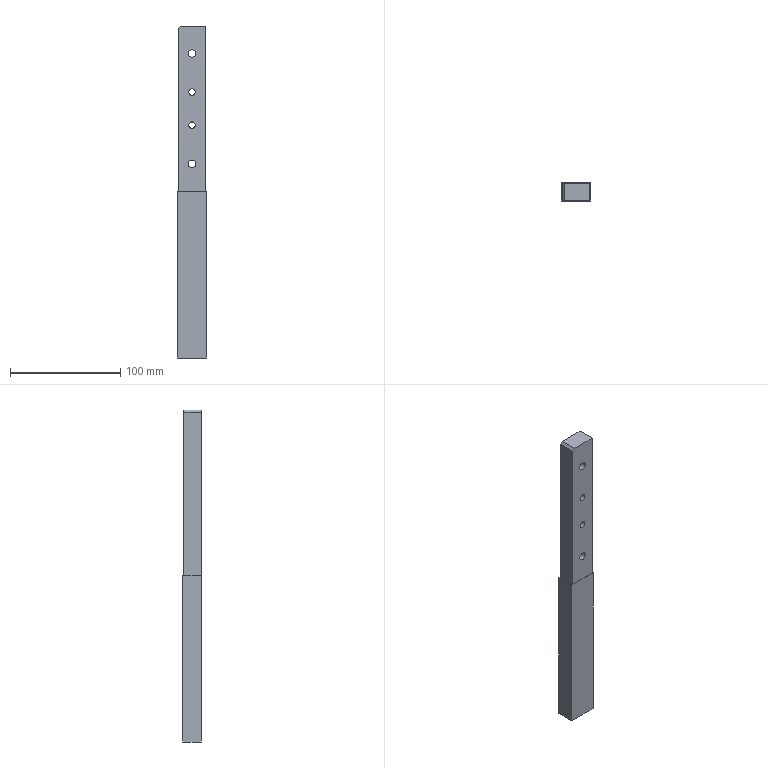Part | NX | features BREP 2 | 2 solids | 25 faces | box 27 x 16.6 x 301 mm | volume 123108 mm3 | plane 17 | cylinder 8 | commonest cylinder face diameters 7 x4 6 x2 11 x2
STEP:
#1=CARTESIAN_POINT('',(26.,16.6,0.));
#2=VERTEX_POINT('',#1);
#3=CARTESIAN_POINT('',(26.,0.,0.));
#4=VERTEX_POINT('',#3);
#5=CARTESIAN_POINT('',(26.,15.6,0.));
#6=DIRECTION('',(0.,-1.,0.));
#7=VECTOR('',#6,1000.);
#8=LINE('',#5,#7);
#9=EDGE_CURVE('',#2,#4,#8,.T.);
#10=ORIENTED_EDGE('',*,*,#9,.T.);
#11=CARTESIAN_POINT('',(26.,0.,-151.));
#12=VERTEX_POINT('',#11);
#13=CARTESIAN_POINT('',(26.,0.,-151.));
#14=DIRECTION('',(0.,0.,1.));
#15=VECTOR('',#14,1000.);
#16=LINE('',#13,#15);
#17=EDGE_CURVE('',#12,#4,#16,.T.);
#18=ORIENTED_EDGE('',*,*,#17,.F.);
#19=CARTESIAN_POINT('',(26.,16.6,-151.));
#20=VERTEX_POINT('',#19);
#21=CARTESIAN_POINT('',(26.,15.6,-151.));
#22=DIRECTION('',(0.,-1.,0.));
#23=VECTOR('',#22,1000.);
#24=LINE('',#21,#23);
#25=EDGE_CURVE('',#20,#12,#24,.T.);
#26=ORIENTED_EDGE('',*,*,#25,.F.);
#27=CARTESIAN_POINT('',(26.,16.6,-151.));
#28=DIRECTION('',(0.,0.,1.));
#29=VECTOR('',#28,1000.);
#30=LINE('',#27,#29);
#31=EDGE_CURVE('',#20,#2,#30,.T.);
#32=ORIENTED_EDGE('',*,*,#31,.T.);
#33=EDGE_LOOP('',(#10,#18,#26,#32));
#34=FACE_BOUND('',#33,.T.);
#35=CARTESIAN_POINT('',(26.,15.6,-151.));
#36=DIRECTION('',(-1.,0.,0.));
#37=DIRECTION('',(0.,1.,0.));
#38=AXIS2_PLACEMENT_3D('',#35,#36,#37);
#39=PLANE('',#38);
#40=ADVANCED_FACE('',(#34),#39,.F.);
#41=CARTESIAN_POINT('',(-1.,0.,0.));
#42=VERTEX_POINT('',#41);
#43=CARTESIAN_POINT('',(25.,0.,0.));
#44=DIRECTION('',(-1.,0.,0.));
#45=VECTOR('',#44,1000.);
#46=LINE('',#43,#45);
#47=EDGE_CURVE('',#4,#42,#46,.T.);
#48=ORIENTED_EDGE('',*,*,#47,.T.);
#49=CARTESIAN_POINT('',(-1.,0.,-151.));
#50=VERTEX_POINT('',#49);
#51=CARTESIAN_POINT('',(-1.,0.,-151.));
#52=DIRECTION('',(0.,0.,1.));
#53=VECTOR('',#52,1000.);
#54=LINE('',#51,#53);
#55=EDGE_CURVE('',#50,#42,#54,.T.);
#56=ORIENTED_EDGE('',*,*,#55,.F.);
#57=CARTESIAN_POINT('',(25.,0.,-151.));
#58=DIRECTION('',(-1.,0.,0.));
#59=VECTOR('',#58,1000.);
#60=LINE('',#57,#59);
#61=EDGE_CURVE('',#12,#50,#60,.T.);
#62=ORIENTED_EDGE('',*,*,#61,.F.);
#63=ORIENTED_EDGE('',*,*,#17,.T.);
#64=EDGE_LOOP('',(#48,#56,#62,#63));
#65=FACE_BOUND('',#64,.T.);
#66=CARTESIAN_POINT('',(25.,0.,-151.));
#67=DIRECTION('',(0.,1.,0.));
#68=DIRECTION('',(1.,0.,0.));
#69=AXIS2_PLACEMENT_3D('',#66,#67,#68);
#70=PLANE('',#69);
#71=ADVANCED_FACE('',(#65),#70,.F.);
#72=CARTESIAN_POINT('',(-1.,16.6,0.));
#73=VERTEX_POINT('',#72);
#74=CARTESIAN_POINT('',(-1.,10.6,0.));
#75=DIRECTION('',(0.,1.,0.));
#76=VECTOR('',#75,1000.);
#77=LINE('',#74,#76);
#78=EDGE_CURVE('',#42,#73,#77,.T.);
#79=ORIENTED_EDGE('',*,*,#78,.T.);
#80=CARTESIAN_POINT('',(-1.,16.6,-151.));
#81=VERTEX_POINT('',#80);
#82=CARTESIAN_POINT('',(-1.,16.6,-151.));
#83=DIRECTION('',(0.,0.,1.));
#84=VECTOR('',#83,1000.);
#85=LINE('',#82,#84);
#86=EDGE_CURVE('',#81,#73,#85,.T.);
#87=ORIENTED_EDGE('',*,*,#86,.F.);
#88=CARTESIAN_POINT('',(-1.,10.6,-151.));
#89=DIRECTION('',(0.,1.,0.));
#90=VECTOR('',#89,1000.);
#91=LINE('',#88,#90);
#92=EDGE_CURVE('',#50,#81,#91,.T.);
#93=ORIENTED_EDGE('',*,*,#92,.F.);
#94=ORIENTED_EDGE('',*,*,#55,.T.);
#95=EDGE_LOOP('',(#79,#87,#93,#94));
#96=FACE_BOUND('',#95,.T.);
#97=CARTESIAN_POINT('',(-1.,10.6,-151.));
#98=DIRECTION('',(1.,0.,0.));
#99=DIRECTION('',(0.,0.,1.));
#100=AXIS2_PLACEMENT_3D('',#97,#98,#99);
#101=PLANE('',#100);
#102=ADVANCED_FACE('',(#96),#101,.F.);
#103=CARTESIAN_POINT('',(0.,16.6,0.));
#104=DIRECTION('',(1.,0.,0.));
#105=VECTOR('',#104,1000.);
#106=LINE('',#103,#105);
#107=EDGE_CURVE('',#73,#2,#106,.T.);
#108=ORIENTED_EDGE('',*,*,#107,.T.);
#109=ORIENTED_EDGE('',*,*,#31,.F.);
#110=CARTESIAN_POINT('',(0.,16.6,-151.));
#111=DIRECTION('',(1.,0.,0.));
#112=VECTOR('',#111,1000.);
#113=LINE('',#110,#112);
#114=EDGE_CURVE('',#81,#20,#113,.T.);
#115=ORIENTED_EDGE('',*,*,#114,.F.);
#116=ORIENTED_EDGE('',*,*,#86,.T.);
#117=EDGE_LOOP('',(#108,#109,#115,#116));
#118=FACE_BOUND('',#117,.T.);
#119=CARTESIAN_POINT('',(0.,16.6,-151.));
#120=DIRECTION('',(0.,-1.,0.));
#121=DIRECTION('',(0.,0.,1.));
#122=AXIS2_PLACEMENT_3D('',#119,#120,#121);
#123=PLANE('',#122);
#124=ADVANCED_FACE('',(#118),#123,.F.);
#125=ORIENTED_EDGE('',*,*,#25,.T.);
#126=ORIENTED_EDGE('',*,*,#61,.T.);
#127=ORIENTED_EDGE('',*,*,#92,.T.);
#128=ORIENTED_EDGE('',*,*,#114,.T.);
#129=EDGE_LOOP('',(#125,#126,#127,#128));
#130=FACE_BOUND('',#129,.T.);
#131=CARTESIAN_POINT('',(25.,0.,-151.));
#132=DIRECTION('',(0.,0.,-1.));
#133=DIRECTION('',(1.,0.,0.));
#134=AXIS2_PLACEMENT_3D('',#131,#132,#133);
#135=PLANE('',#134);
#136=ADVANCED_FACE('',(#130),#135,.T.);
#137=ORIENTED_EDGE('',*,*,#9,.F.);
#138=ORIENTED_EDGE('',*,*,#107,.F.);
#139=ORIENTED_EDGE('',*,*,#78,.F.);
#140=ORIENTED_EDGE('',*,*,#47,.F.);
#141=EDGE_LOOP('',(#137,#138,#139,#140));
#142=FACE_BOUND('',#141,.T.);
#143=CARTESIAN_POINT('',(25.,0.,0.));
#144=DIRECTION('',(0.,0.,-1.));
#145=DIRECTION('',(1.,0.,0.));
#146=AXIS2_PLACEMENT_3D('',#143,#144,#145);
#147=PLANE('',#146);
#148=ADVANCED_FACE('',(#142),#147,.F.);
#149=CLOSED_SHELL('',(#40,#71,#102,#124,#136,#148));
#150=MANIFOLD_SOLID_BREP('',#149);
#151=CARTESIAN_POINT('',(25.,0.,150.));
#152=VERTEX_POINT('',#151);
#153=CARTESIAN_POINT('',(25.,0.,0.));
#154=VERTEX_POINT('',#153);
#155=CARTESIAN_POINT('',(25.,0.,150.));
#156=DIRECTION('',(0.,0.,-1.));
#157=VECTOR('',#156,1000.);
#158=LINE('',#155,#157);
#159=EDGE_CURVE('',#152,#154,#158,.T.);
#160=ORIENTED_EDGE('',*,*,#159,.T.);
#161=CARTESIAN_POINT('',(25.,15.6,0.));
#162=VERTEX_POINT('',#161);
#163=CARTESIAN_POINT('',(25.,15.6,0.));
#164=DIRECTION('',(0.,1.,0.));
#165=VECTOR('',#164,1000.);
#166=LINE('',#163,#165);
#167=EDGE_CURVE('',#154,#162,#166,.T.);
#168=ORIENTED_EDGE('',*,*,#167,.T.);
#169=CARTESIAN_POINT('',(25.,15.6,150.));
#170=VERTEX_POINT('',#169);
#171=CARTESIAN_POINT('',(25.,15.6,150.));
#172=DIRECTION('',(0.,0.,-1.));
#173=VECTOR('',#172,1000.);
#174=LINE('',#171,#173);
#175=EDGE_CURVE('',#170,#162,#174,.T.);
#176=ORIENTED_EDGE('',*,*,#175,.F.);
#177=CARTESIAN_POINT('',(25.,15.6,150.));
#178=DIRECTION('',(0.,-1.,0.));
#179=VECTOR('',#178,1000.);
#180=LINE('',#177,#179);
#181=EDGE_CURVE('',#170,#152,#180,.T.);
#182=ORIENTED_EDGE('',*,*,#181,.T.);
#183=EDGE_LOOP('',(#160,#168,#176,#182));
#184=FACE_BOUND('',#183,.T.);
#185=CARTESIAN_POINT('',(25.,15.6,150.));
#186=DIRECTION('',(1.,0.,0.));
#187=DIRECTION('',(0.,-1.,0.));
#188=AXIS2_PLACEMENT_3D('',#185,#186,#187);
#189=PLANE('',#188);
#190=ADVANCED_FACE('',(#184),#189,.T.);
#191=CARTESIAN_POINT('',(0.,15.6,148.));
#192=VERTEX_POINT('',#191);
#193=CARTESIAN_POINT('',(0.,15.6,0.));
#194=VERTEX_POINT('',#193);
#195=CARTESIAN_POINT('',(0.,15.6,150.));
#196=DIRECTION('',(0.,0.,-1.));
#197=VECTOR('',#196,1000.);
#198=LINE('',#195,#197);
#199=EDGE_CURVE('',#192,#194,#198,.T.);
#200=ORIENTED_EDGE('',*,*,#199,.T.);
#201=CARTESIAN_POINT('',(0.,0.,0.));
#202=VERTEX_POINT('',#201);
#203=CARTESIAN_POINT('',(0.,10.6,0.));
#204=DIRECTION('',(0.,-1.,0.));
#205=VECTOR('',#204,1000.);
#206=LINE('',#203,#205);
#207=EDGE_CURVE('',#194,#202,#206,.T.);
#208=ORIENTED_EDGE('',*,*,#207,.T.);
#209=CARTESIAN_POINT('',(0.,0.,148.));
#210=VERTEX_POINT('',#209);
#211=CARTESIAN_POINT('',(0.,0.,150.));
#212=DIRECTION('',(0.,0.,-1.));
#213=VECTOR('',#212,1000.);
#214=LINE('',#211,#213);
#215=EDGE_CURVE('',#210,#202,#214,.T.);
#216=ORIENTED_EDGE('',*,*,#215,.F.);
#217=CARTESIAN_POINT('',(0.,15.6,148.));
#218=DIRECTION('',(0.,1.,0.));
#219=VECTOR('',#218,1000.);
#220=LINE('',#217,#219);
#221=EDGE_CURVE('',#210,#192,#220,.T.);
#222=ORIENTED_EDGE('',*,*,#221,.T.);
#223=EDGE_LOOP('',(#200,#208,#216,#222));
#224=FACE_BOUND('',#223,.T.);
#225=CARTESIAN_POINT('',(0.,10.6,150.));
#226=DIRECTION('',(-1.,0.,0.));
#227=DIRECTION('',(0.,0.,-1.));
#228=AXIS2_PLACEMENT_3D('',#225,#226,#227);
#229=PLANE('',#228);
#230=ADVANCED_FACE('',(#224),#229,.T.);
#231=CARTESIAN_POINT('',(12.5,15.6,86.5));
#232=VERTEX_POINT('',#231);
#233=CARTESIAN_POINT('',(12.5,15.6,90.));
#234=DIRECTION('',(0.,1.,0.));
#235=DIRECTION('',(0.,0.,-1.));
#236=AXIS2_PLACEMENT_3D('',#233,#234,#235);
#237=CIRCLE('',#236,3.5);
#238=EDGE_CURVE('',#232,#232,#237,.T.);
#239=ORIENTED_EDGE('',*,*,#238,.F.);
#240=EDGE_LOOP('',(#239));
#241=FACE_BOUND('',#240,.T.);
#242=CARTESIAN_POINT('',(12.5,15.6,56.5));
#243=VERTEX_POINT('',#242);
#244=CARTESIAN_POINT('',(12.5,15.6,60.));
#245=DIRECTION('',(0.,1.,0.));
#246=DIRECTION('',(0.,0.,-1.));
#247=AXIS2_PLACEMENT_3D('',#244,#245,#246);
#248=CIRCLE('',#247,3.5);
#249=EDGE_CURVE('',#243,#243,#248,.T.);
#250=ORIENTED_EDGE('',*,*,#249,.F.);
#251=EDGE_LOOP('',(#250));
#252=FACE_BOUND('',#251,.T.);
#253=CARTESIAN_POINT('',(12.5,15.6,119.5));
#254=VERTEX_POINT('',#253);
#255=CARTESIAN_POINT('',(12.5,15.6,125.));
#256=DIRECTION('',(0.,1.,0.));
#257=DIRECTION('',(0.,0.,-1.));
#258=AXIS2_PLACEMENT_3D('',#255,#256,#257);
#259=CIRCLE('',#258,5.5);
#260=EDGE_CURVE('',#254,#254,#259,.T.);
#261=ORIENTED_EDGE('',*,*,#260,.F.);
#262=EDGE_LOOP('',(#261));
#263=FACE_BOUND('',#262,.T.);
#264=CARTESIAN_POINT('',(12.5,15.6,19.5));
#265=VERTEX_POINT('',#264);
#266=CARTESIAN_POINT('',(12.5,15.6,25.));
#267=DIRECTION('',(0.,1.,0.));
#268=DIRECTION('',(0.,0.,-1.));
#269=AXIS2_PLACEMENT_3D('',#266,#267,#268);
#270=CIRCLE('',#269,5.5);
#271=EDGE_CURVE('',#265,#265,#270,.T.);
#272=ORIENTED_EDGE('',*,*,#271,.F.);
#273=EDGE_LOOP('',(#272));
#274=FACE_BOUND('',#273,.T.);
#275=ORIENTED_EDGE('',*,*,#175,.T.);
#276=CARTESIAN_POINT('',(0.,15.6,0.));
#277=DIRECTION('',(-1.,0.,0.));
#278=VECTOR('',#277,1000.);
#279=LINE('',#276,#278);
#280=EDGE_CURVE('',#162,#194,#279,.T.);
#281=ORIENTED_EDGE('',*,*,#280,.T.);
#282=ORIENTED_EDGE('',*,*,#199,.F.);
#283=CARTESIAN_POINT('',(2.,15.6,150.));
#284=VERTEX_POINT('',#283);
#285=CARTESIAN_POINT('',(1.,15.6,149.));
#286=DIRECTION('',(0.7071,0.,0.7071));
#287=VECTOR('',#286,1000.);
#288=LINE('',#285,#287);
#289=EDGE_CURVE('',#192,#284,#288,.T.);
#290=ORIENTED_EDGE('',*,*,#289,.T.);
#291=CARTESIAN_POINT('',(0.,15.6,150.));
#292=DIRECTION('',(1.,0.,0.));
#293=VECTOR('',#292,1000.);
#294=LINE('',#291,#293);
#295=EDGE_CURVE('',#284,#170,#294,.T.);
#296=ORIENTED_EDGE('',*,*,#295,.T.);
#297=EDGE_LOOP('',(#275,#281,#282,#290,#296));
#298=FACE_BOUND('',#297,.T.);
#299=CARTESIAN_POINT('',(0.,15.6,150.));
#300=DIRECTION('',(0.,1.,0.));
#301=DIRECTION('',(0.,0.,-1.));
#302=AXIS2_PLACEMENT_3D('',#299,#300,#301);
#303=PLANE('',#302);
#304=ADVANCED_FACE('',(#241,#252,#263,#274,#298),#303,.T.);
#305=CARTESIAN_POINT('',(15.5,0.,90.));
#306=VERTEX_POINT('',#305);
#307=CARTESIAN_POINT('',(12.5,0.,90.));
#308=DIRECTION('',(0.,-1.,0.));
#309=DIRECTION('',(1.,0.,0.));
#310=AXIS2_PLACEMENT_3D('',#307,#308,#309);
#311=CIRCLE('',#310,3.);
#312=EDGE_CURVE('',#306,#306,#311,.T.);
#313=ORIENTED_EDGE('',*,*,#312,.F.);
#314=EDGE_LOOP('',(#313));
#315=FACE_BOUND('',#314,.T.);
#316=CARTESIAN_POINT('',(15.5,0.,60.));
#317=VERTEX_POINT('',#316);
#318=CARTESIAN_POINT('',(12.5,0.,60.));
#319=DIRECTION('',(0.,-1.,0.));
#320=DIRECTION('',(1.,0.,0.));
#321=AXIS2_PLACEMENT_3D('',#318,#319,#320);
#322=CIRCLE('',#321,3.);
#323=EDGE_CURVE('',#317,#317,#322,.T.);
#324=ORIENTED_EDGE('',*,*,#323,.F.);
#325=EDGE_LOOP('',(#324));
#326=FACE_BOUND('',#325,.T.);
#327=CARTESIAN_POINT('',(12.5,0.,128.5));
#328=VERTEX_POINT('',#327);
#329=CARTESIAN_POINT('',(12.5,0.,125.));
#330=DIRECTION('',(0.,-1.,0.));
#331=DIRECTION('',(0.,0.,1.));
#332=AXIS2_PLACEMENT_3D('',#329,#330,#331);
#333=CIRCLE('',#332,3.5);
#334=EDGE_CURVE('',#328,#328,#333,.T.);
#335=ORIENTED_EDGE('',*,*,#334,.F.);
#336=EDGE_LOOP('',(#335));
#337=FACE_BOUND('',#336,.T.);
#338=CARTESIAN_POINT('',(12.5,0.,28.5));
#339=VERTEX_POINT('',#338);
#340=CARTESIAN_POINT('',(12.5,0.,25.));
#341=DIRECTION('',(0.,-1.,0.));
#342=DIRECTION('',(0.,0.,1.));
#343=AXIS2_PLACEMENT_3D('',#340,#341,#342);
#344=CIRCLE('',#343,3.5);
#345=EDGE_CURVE('',#339,#339,#344,.T.);
#346=ORIENTED_EDGE('',*,*,#345,.F.);
#347=EDGE_LOOP('',(#346));
#348=FACE_BOUND('',#347,.T.);
#349=CARTESIAN_POINT('',(25.,0.,0.));
#350=DIRECTION('',(-1.,0.,0.));
#351=VECTOR('',#350,1000.);
#352=LINE('',#349,#351);
#353=EDGE_CURVE('',#154,#202,#352,.T.);
#354=ORIENTED_EDGE('',*,*,#353,.F.);
#355=ORIENTED_EDGE('',*,*,#159,.F.);
#356=CARTESIAN_POINT('',(2.,0.,150.));
#357=VERTEX_POINT('',#356);
#358=CARTESIAN_POINT('',(25.,0.,150.));
#359=DIRECTION('',(-1.,0.,0.));
#360=VECTOR('',#359,1000.);
#361=LINE('',#358,#360);
#362=EDGE_CURVE('',#152,#357,#361,.T.);
#363=ORIENTED_EDGE('',*,*,#362,.T.);
#364=CARTESIAN_POINT('',(13.5,0.,161.5));
#365=DIRECTION('',(-0.7071,0.,-0.7071));
#366=VECTOR('',#365,1000.);
#367=LINE('',#364,#366);
#368=EDGE_CURVE('',#357,#210,#367,.T.);
#369=ORIENTED_EDGE('',*,*,#368,.T.);
#370=ORIENTED_EDGE('',*,*,#215,.T.);
#371=EDGE_LOOP('',(#354,#355,#363,#369,#370));
#372=FACE_BOUND('',#371,.T.);
#373=CARTESIAN_POINT('',(25.,0.,150.));
#374=DIRECTION('',(0.,-1.,0.));
#375=DIRECTION('',(-1.,0.,0.));
#376=AXIS2_PLACEMENT_3D('',#373,#374,#375);
#377=PLANE('',#376);
#378=ADVANCED_FACE('',(#315,#326,#337,#348,#372),#377,.T.);
#379=ORIENTED_EDGE('',*,*,#295,.F.);
#380=CARTESIAN_POINT('',(2.,0.,150.));
#381=DIRECTION('',(0.,-1.,0.));
#382=VECTOR('',#381,1000.);
#383=LINE('',#380,#382);
#384=EDGE_CURVE('',#284,#357,#383,.T.);
#385=ORIENTED_EDGE('',*,*,#384,.T.);
#386=ORIENTED_EDGE('',*,*,#362,.F.);
#387=ORIENTED_EDGE('',*,*,#181,.F.);
#388=EDGE_LOOP('',(#379,#385,#386,#387));
#389=FACE_BOUND('',#388,.T.);
#390=CARTESIAN_POINT('',(25.,0.,150.));
#391=DIRECTION('',(0.,0.,-1.));
#392=DIRECTION('',(1.,0.,0.));
#393=AXIS2_PLACEMENT_3D('',#390,#391,#392);
#394=PLANE('',#393);
#395=ADVANCED_FACE('',(#389),#394,.F.);
#396=ORIENTED_EDGE('',*,*,#368,.F.);
#397=ORIENTED_EDGE('',*,*,#384,.F.);
#398=ORIENTED_EDGE('',*,*,#289,.F.);
#399=ORIENTED_EDGE('',*,*,#221,.F.);
#400=EDGE_LOOP('',(#396,#397,#398,#399));
#401=FACE_BOUND('',#400,.T.);
#402=CARTESIAN_POINT('',(0.,10.6,148.));
#403=DIRECTION('',(-0.7071,0.,0.7071));
#404=DIRECTION('',(-0.7071,0.,-0.7071));
#405=AXIS2_PLACEMENT_3D('',#402,#403,#404);
#406=PLANE('',#405);
#407=ADVANCED_FACE('',(#401),#406,.T.);
#408=ORIENTED_EDGE('',*,*,#353,.T.);
#409=ORIENTED_EDGE('',*,*,#207,.F.);
#410=ORIENTED_EDGE('',*,*,#280,.F.);
#411=ORIENTED_EDGE('',*,*,#167,.F.);
#412=EDGE_LOOP('',(#408,#409,#410,#411));
#413=FACE_BOUND('',#412,.T.);
#414=CARTESIAN_POINT('',(25.,0.,0.));
#415=DIRECTION('',(0.,0.,-1.));
#416=DIRECTION('',(1.,0.,0.));
#417=AXIS2_PLACEMENT_3D('',#414,#415,#416);
#418=PLANE('',#417);
#419=ADVANCED_FACE('',(#413),#418,.T.);
#420=ORIENTED_EDGE('',*,*,#345,.T.);
#421=EDGE_LOOP('',(#420));
#422=FACE_BOUND('',#421,.T.);
#423=CARTESIAN_POINT('',(12.5,7.6,28.5));
#424=VERTEX_POINT('',#423);
#425=CARTESIAN_POINT('',(12.5,7.6,25.));
#426=DIRECTION('',(0.,1.,0.));
#427=DIRECTION('',(0.,0.,1.));
#428=AXIS2_PLACEMENT_3D('',#425,#426,#427);
#429=CIRCLE('',#428,3.5);
#430=EDGE_CURVE('',#424,#424,#429,.T.);
#431=ORIENTED_EDGE('',*,*,#430,.T.);
#432=EDGE_LOOP('',(#431));
#433=FACE_BOUND('',#432,.T.);
#434=CARTESIAN_POINT('',(12.5,7.6,25.));
#435=DIRECTION('',(0.,-1.,0.));
#436=DIRECTION('',(0.,0.,-1.));
#437=AXIS2_PLACEMENT_3D('',#434,#435,#436);
#438=CYLINDRICAL_SURFACE('',#437,3.5);
#439=ADVANCED_FACE('',(#422,#433),#438,.F.);
#440=ORIENTED_EDGE('',*,*,#271,.T.);
#441=EDGE_LOOP('',(#440));
#442=FACE_BOUND('',#441,.T.);
#443=CARTESIAN_POINT('',(12.5,7.6,19.5));
#444=VERTEX_POINT('',#443);
#445=CARTESIAN_POINT('',(12.5,7.6,25.));
#446=DIRECTION('',(0.,-1.,0.));
#447=DIRECTION('',(0.,0.,-1.));
#448=AXIS2_PLACEMENT_3D('',#445,#446,#447);
#449=CIRCLE('',#448,5.5);
#450=EDGE_CURVE('',#444,#444,#449,.T.);
#451=ORIENTED_EDGE('',*,*,#450,.T.);
#452=EDGE_LOOP('',(#451));
#453=FACE_BOUND('',#452,.T.);
#454=CARTESIAN_POINT('',(12.5,7.6,25.));
#455=DIRECTION('',(0.,1.,0.));
#456=DIRECTION('',(0.,0.,1.));
#457=AXIS2_PLACEMENT_3D('',#454,#455,#456);
#458=CYLINDRICAL_SURFACE('',#457,5.5);
#459=ADVANCED_FACE('',(#442,#453),#458,.F.);
#460=ORIENTED_EDGE('',*,*,#430,.F.);
#461=EDGE_LOOP('',(#460));
#462=FACE_BOUND('',#461,.T.);
#463=ORIENTED_EDGE('',*,*,#450,.F.);
#464=EDGE_LOOP('',(#463));
#465=FACE_BOUND('',#464,.T.);
#466=CARTESIAN_POINT('',(12.5,7.6,25.));
#467=DIRECTION('',(0.,-1.,0.));
#468=DIRECTION('',(0.,0.,-1.));
#469=AXIS2_PLACEMENT_3D('',#466,#467,#468);
#470=PLANE('',#469);
#471=ADVANCED_FACE('',(#462,#465),#470,.F.);
#472=ORIENTED_EDGE('',*,*,#334,.T.);
#473=EDGE_LOOP('',(#472));
#474=FACE_BOUND('',#473,.T.);
#475=CARTESIAN_POINT('',(12.5,7.6,128.5));
#476=VERTEX_POINT('',#475);
#477=CARTESIAN_POINT('',(12.5,7.6,125.));
#478=DIRECTION('',(0.,1.,0.));
#479=DIRECTION('',(0.,0.,1.));
#480=AXIS2_PLACEMENT_3D('',#477,#478,#479);
#481=CIRCLE('',#480,3.5);
#482=EDGE_CURVE('',#476,#476,#481,.T.);
#483=ORIENTED_EDGE('',*,*,#482,.T.);
#484=EDGE_LOOP('',(#483));
#485=FACE_BOUND('',#484,.T.);
#486=CARTESIAN_POINT('',(12.5,7.6,125.));
#487=DIRECTION('',(0.,-1.,0.));
#488=DIRECTION('',(0.,0.,-1.));
#489=AXIS2_PLACEMENT_3D('',#486,#487,#488);
#490=CYLINDRICAL_SURFACE('',#489,3.5);
#491=ADVANCED_FACE('',(#474,#485),#490,.F.);
#492=ORIENTED_EDGE('',*,*,#260,.T.);
#493=EDGE_LOOP('',(#492));
#494=FACE_BOUND('',#493,.T.);
#495=CARTESIAN_POINT('',(12.5,7.6,119.5));
#496=VERTEX_POINT('',#495);
#497=CARTESIAN_POINT('',(12.5,7.6,125.));
#498=DIRECTION('',(0.,-1.,0.));
#499=DIRECTION('',(0.,0.,-1.));
#500=AXIS2_PLACEMENT_3D('',#497,#498,#499);
#501=CIRCLE('',#500,5.5);
#502=EDGE_CURVE('',#496,#496,#501,.T.);
#503=ORIENTED_EDGE('',*,*,#502,.T.);
#504=EDGE_LOOP('',(#503));
#505=FACE_BOUND('',#504,.T.);
#506=CARTESIAN_POINT('',(12.5,7.6,125.));
#507=DIRECTION('',(0.,1.,0.));
#508=DIRECTION('',(0.,0.,1.));
#509=AXIS2_PLACEMENT_3D('',#506,#507,#508);
#510=CYLINDRICAL_SURFACE('',#509,5.5);
#511=ADVANCED_FACE('',(#494,#505),#510,.F.);
#512=ORIENTED_EDGE('',*,*,#482,.F.);
#513=EDGE_LOOP('',(#512));
#514=FACE_BOUND('',#513,.T.);
#515=ORIENTED_EDGE('',*,*,#502,.F.);
#516=EDGE_LOOP('',(#515));
#517=FACE_BOUND('',#516,.T.);
#518=CARTESIAN_POINT('',(12.5,7.6,125.));
#519=DIRECTION('',(0.,-1.,0.));
#520=DIRECTION('',(0.,0.,-1.));
#521=AXIS2_PLACEMENT_3D('',#518,#519,#520);
#522=PLANE('',#521);
#523=ADVANCED_FACE('',(#514,#517),#522,.F.);
#524=CARTESIAN_POINT('',(12.5,13.1,56.5));
#525=VERTEX_POINT('',#524);
#526=CARTESIAN_POINT('',(12.5,13.1,60.));
#527=DIRECTION('',(0.,-1.,0.));
#528=DIRECTION('',(0.,0.,-1.));
#529=AXIS2_PLACEMENT_3D('',#526,#527,#528);
#530=CIRCLE('',#529,3.5);
#531=EDGE_CURVE('',#525,#525,#530,.T.);
#532=ORIENTED_EDGE('',*,*,#531,.T.);
#533=EDGE_LOOP('',(#532));
#534=FACE_BOUND('',#533,.T.);
#535=ORIENTED_EDGE('',*,*,#249,.T.);
#536=EDGE_LOOP('',(#535));
#537=FACE_BOUND('',#536,.T.);
#538=CARTESIAN_POINT('',(12.5,13.1,60.));
#539=DIRECTION('',(0.,1.,0.));
#540=DIRECTION('',(0.,0.,1.));
#541=AXIS2_PLACEMENT_3D('',#538,#539,#540);
#542=CYLINDRICAL_SURFACE('',#541,3.5);
#543=ADVANCED_FACE('',(#534,#537),#542,.F.);
#544=CARTESIAN_POINT('',(12.5,13.1,63.));
#545=VERTEX_POINT('',#544);
#546=CARTESIAN_POINT('',(12.5,13.1,60.));
#547=DIRECTION('',(0.,1.,0.));
#548=DIRECTION('',(0.,0.,1.));
#549=AXIS2_PLACEMENT_3D('',#546,#547,#548);
#550=CIRCLE('',#549,3.);
#551=EDGE_CURVE('',#545,#545,#550,.T.);
#552=ORIENTED_EDGE('',*,*,#551,.F.);
#553=EDGE_LOOP('',(#552));
#554=FACE_BOUND('',#553,.T.);
#555=ORIENTED_EDGE('',*,*,#531,.F.);
#556=EDGE_LOOP('',(#555));
#557=FACE_BOUND('',#556,.T.);
#558=CARTESIAN_POINT('',(12.5,13.1,60.));
#559=DIRECTION('',(0.,1.,0.));
#560=DIRECTION('',(0.,0.,1.));
#561=AXIS2_PLACEMENT_3D('',#558,#559,#560);
#562=PLANE('',#561);
#563=ADVANCED_FACE('',(#554,#557),#562,.T.);
#564=ORIENTED_EDGE('',*,*,#323,.T.);
#565=EDGE_LOOP('',(#564));
#566=FACE_BOUND('',#565,.T.);
#567=ORIENTED_EDGE('',*,*,#551,.T.);
#568=EDGE_LOOP('',(#567));
#569=FACE_BOUND('',#568,.T.);
#570=CARTESIAN_POINT('',(12.5,13.1,60.));
#571=DIRECTION('',(0.,-1.,0.));
#572=DIRECTION('',(0.,0.,-1.));
#573=AXIS2_PLACEMENT_3D('',#570,#571,#572);
#574=CYLINDRICAL_SURFACE('',#573,3.);
#575=ADVANCED_FACE('',(#566,#569),#574,.F.);
#576=CARTESIAN_POINT('',(12.5,13.1,86.5));
#577=VERTEX_POINT('',#576);
#578=CARTESIAN_POINT('',(12.5,13.1,90.));
#579=DIRECTION('',(0.,-1.,0.));
#580=DIRECTION('',(0.,0.,-1.));
#581=AXIS2_PLACEMENT_3D('',#578,#579,#580);
#582=CIRCLE('',#581,3.5);
#583=EDGE_CURVE('',#577,#577,#582,.T.);
#584=ORIENTED_EDGE('',*,*,#583,.T.);
#585=EDGE_LOOP('',(#584));
#586=FACE_BOUND('',#585,.T.);
#587=ORIENTED_EDGE('',*,*,#238,.T.);
#588=EDGE_LOOP('',(#587));
#589=FACE_BOUND('',#588,.T.);
#590=CARTESIAN_POINT('',(12.5,13.1,90.));
#591=DIRECTION('',(0.,1.,0.));
#592=DIRECTION('',(0.,0.,1.));
#593=AXIS2_PLACEMENT_3D('',#590,#591,#592);
#594=CYLINDRICAL_SURFACE('',#593,3.5);
#595=ADVANCED_FACE('',(#586,#589),#594,.F.);
#596=CARTESIAN_POINT('',(12.5,13.1,93.));
#597=VERTEX_POINT('',#596);
#598=CARTESIAN_POINT('',(12.5,13.1,90.));
#599=DIRECTION('',(0.,1.,0.));
#600=DIRECTION('',(0.,0.,1.));
#601=AXIS2_PLACEMENT_3D('',#598,#599,#600);
#602=CIRCLE('',#601,3.);
#603=EDGE_CURVE('',#597,#597,#602,.T.);
#604=ORIENTED_EDGE('',*,*,#603,.F.);
#605=EDGE_LOOP('',(#604));
#606=FACE_BOUND('',#605,.T.);
#607=ORIENTED_EDGE('',*,*,#583,.F.);
#608=EDGE_LOOP('',(#607));
#609=FACE_BOUND('',#608,.T.);
#610=CARTESIAN_POINT('',(12.5,13.1,90.));
#611=DIRECTION('',(0.,1.,0.));
#612=DIRECTION('',(0.,0.,1.));
#613=AXIS2_PLACEMENT_3D('',#610,#611,#612);
#614=PLANE('',#613);
#615=ADVANCED_FACE('',(#606,#609),#614,.T.);
#616=ORIENTED_EDGE('',*,*,#312,.T.);
#617=EDGE_LOOP('',(#616));
#618=FACE_BOUND('',#617,.T.);
#619=ORIENTED_EDGE('',*,*,#603,.T.);
#620=EDGE_LOOP('',(#619));
#621=FACE_BOUND('',#620,.T.);
#622=CARTESIAN_POINT('',(12.5,13.1,90.));
#623=DIRECTION('',(0.,-1.,0.));
#624=DIRECTION('',(0.,0.,-1.));
#625=AXIS2_PLACEMENT_3D('',#622,#623,#624);
#626=CYLINDRICAL_SURFACE('',#625,3.);
#627=ADVANCED_FACE('',(#618,#621),#626,.F.);
#628=CLOSED_SHELL('',(#190,#230,#304,#378,#395,#407,#419,#439,#459,#471,#491,#511,#523,#543,#563,#575,#595,#615,#627));
#629=MANIFOLD_SOLID_BREP('',#628);
#630=(LENGTH_UNIT()NAMED_UNIT(*)SI_UNIT(.MILLI.,.METRE.));
#631=UNCERTAINTY_MEASURE_WITH_UNIT(LENGTH_MEASURE(0.00001),#630,'','');
#632=(NAMED_UNIT(*)PLANE_ANGLE_UNIT()SI_UNIT($,.RADIAN.));
#633=(NAMED_UNIT(*)SI_UNIT($,.STERADIAN.)SOLID_ANGLE_UNIT());
#634=(GEOMETRIC_REPRESENTATION_CONTEXT(3)GLOBAL_UNCERTAINTY_ASSIGNED_CONTEXT((#631))GLOBAL_UNIT_ASSIGNED_CONTEXT((#630,#632,#633))REPRESENTATION_CONTEXT('',''));
#635=ADVANCED_BREP_SHAPE_REPRESENTATION('',(#150,#629),#634);